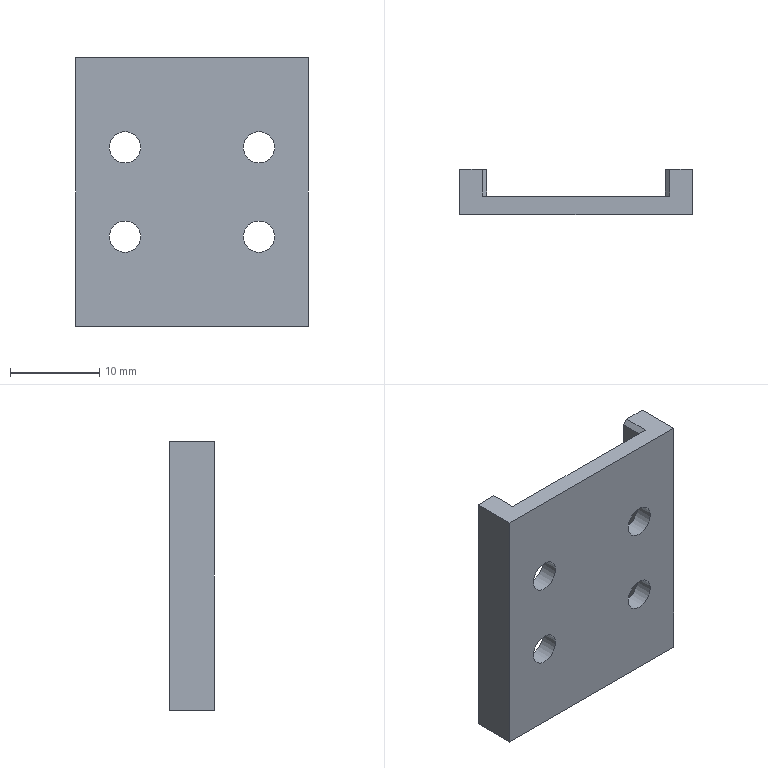NC program | NX | posted with a generic post | part box 26 x 5 x 30 mm
Whole program:
N10 G17 G21 G94 G90
(FLOOR_WALL , TOOL : D50)
N12 T01 M6
N14 G54
N16 G17 G0 G90 X-43. Y0. B0. C0. S2000 M3
N18 G43 Z30. H1
N20 Z3.
N22 G94 G1 Z0. F800.
N24 X-40.
N26 X40.
N28 X43.
N30 Z3.
N32 G0 Z30.
N34 M5
(DRILLING , TOOL : ZXZ)
N36 T02 M6
N38 G54
N40 G17 G0 G90 X-5. Y7.5 B0. C0. S3500 M3
N42 G43 Z30. H2
N44 G94 G81 G98 Z-1. F250. R3.
N46 X5.
N48 Y-7.5
N50 X-5.
N52 G80
N54 G0 X-5. Y-7.5 Z30.
N56 M5
(DRILLING_COPY , TOOL : 3.5ZT)
N58 T13 M6
N60 G54
N62 G17 G0 G90 X-5. Y7.5 B0. C0. S2000 M3
N64 G43 Z30. H13
N66 G94 G83 G98 Z-7.552 F150. Q2. R3.
N68 X5.
N70 Y-7.5
N72 X-5.
N74 G80
N76 G0 X-5. Y-7.5 Z30.
N78 M5
(FLOOR_WALL_1 , TOOL : D10)
N80 T10 M6
N82 G54
N84 G17 G0 G90 X-21.5 Y-1.443 B0. C0. S3000 M3
N86 G43 Z30. H10
N88 Z0.924
N90 G94 G1 Z-0.076 F1000.
N92 X-20.5 Y-0.866
N94 G3 X-20. Y0. R1.
N96 G1 Y8.358 F2000.
N98 X-16.592 Y4.95
N100 X16.592
N102 X20. Y8.358
N104 Y-8.358
N106 X16.592 Y-4.95
N108 X-16.592
N110 X-20. Y-8.358
N112 Y0.
N114 X-15.5
N116 Y0.45
N118 X15.5
N120 Y-0.45
N122 X-15.5
N124 Y0.
N126 G3 X-16. Y0.866 R1.
N128 G1 Z0.924
N130 G0 X-21.5 Y-1.443 Z0.734
N132 G1 Z-0.266 F1000.
N134 X-20.5 Y-0.866
N136 G3 X-20. Y0. R1.
N138 G1 Y8.358 F2000.
N140 X-16.592 Y4.95
N142 X16.592
N144 X20. Y8.358
N146 Y-8.358
N148 X16.592 Y-4.95
N150 X-16.592
N152 X-20. Y-8.358
N154 Y0.
N156 X-15.5
N158 Y0.45
N160 X15.5
N162 Y-0.45
N164 X-15.5
N166 Y0.
N168 G3 X-16. Y0.866 R1.
N170 G1 Z0.734
N172 G0 X-21.5 Y-1.443 Z0.543
N174 G1 Z-0.457 F1000.
N176 X-20.5 Y-0.866
N178 G3 X-20. Y0. R1.
N180 G1 Y8.358 F2000.
N182 X-16.592 Y4.95
N184 X16.592
N186 X20. Y8.358
N188 Y-8.358
N190 X16.592 Y-4.95
N192 X-16.592
N194 X-20. Y-8.358
N196 Y0.
N198 X-15.5
N200 Y0.45
N202 X15.5
N204 Y-0.45
N206 X-15.5
N208 Y0.
N210 G3 X-16. Y0.866 R1.
N212 G1 Z0.543
N214 G0 X-21.5 Y-1.443 Z0.353
N216 G1 Z-0.648 F1000.
N218 X-20.5 Y-0.866
N220 G3 X-20. Y0. R1.
N222 G1 Y8.358 F2000.
N224 X-16.592 Y4.95
N226 X16.592
N228 X20. Y8.358
N230 Y-8.358
N232 X16.592 Y-4.95
N234 X-16.592
N236 X-20. Y-8.358
N238 Y0.
N240 X-15.5
N242 Y0.45
N244 X15.5
N246 Y-0.45
N248 X-15.5
N250 Y0.
N252 G3 X-16. Y0.866 R1.
N254 G1 Z0.353
N256 G0 X-21.5 Y-1.443 Z0.162
N258 G1 Z-0.838 F1000.
N260 X-20.5 Y-0.866
N262 G3 X-20. Y0. R1.
N264 G1 Y8.358 F2000.
N266 X-16.592 Y4.95
N268 X16.592
N270 X20. Y8.358
N272 Y-8.358
N274 X16.592 Y-4.95
N276 X-16.592
N278 X-20. Y-8.358
N280 Y0.
N282 X-15.5
N284 Y0.45
N286 X15.5
N288 Y-0.45
N290 X-15.5
N292 Y0.
N294 G3 X-16. Y0.866 R1.
N296 G1 Z0.162
N298 G0 X-21.5 Y-1.443 Z-0.029
N300 G1 Z-1.029 F1000.
N302 X-20.5 Y-0.866
N304 G3 X-20. Y0. R1.
N306 G1 Y8.358 F2000.
N308 X-16.592 Y4.95
N310 X16.592
N312 X20. Y8.358
N314 Y-8.358
N316 X16.592 Y-4.95
N318 X-16.592
N320 X-20. Y-8.358
N322 Y0.
N324 X-15.5
N326 Y0.45
N328 X15.5
N330 Y-0.45
N332 X-15.5
N334 Y0.
N336 G3 X-16. Y0.866 R1.
N338 G1 Z-0.029
N340 G0 X-21.5 Y-1.443 Z-0.219
N342 G1 Z-1.219 F1000.
N344 X-20.5 Y-0.866
N346 G3 X-20. Y0. R1.
N348 G1 Y8.358 F2000.
N350 X-16.592 Y4.95
N352 X16.592
N354 X20. Y8.358
N356 Y-8.358
N358 X16.592 Y-4.95
N360 X-16.592
N362 X-20. Y-8.358
N364 Y0.
N366 X-15.5
N368 Y0.45
N370 X15.5
N372 Y-0.45
N374 X-15.5
N376 Y0.
N378 G3 X-16. Y0.866 R1.
N380 G1 Z-0.219
N382 G0 X-21.5 Y-1.443 Z-0.41
N384 G1 Z-1.41 F1000.
N386 X-20.5 Y-0.866
N388 G3 X-20. Y0. R1.
N390 G1 Y8.358 F2000.
N392 X-16.592 Y4.95
N394 X16.592
N396 X20. Y8.358
N398 Y-8.358
N400 X16.592 Y-4.95
N402 X-16.592
N404 X-20. Y-8.358
N406 Y0.
N408 X-15.5
N410 Y0.45
N412 X15.5
N414 Y-0.45
N416 X-15.5
N418 Y0.
N420 G3 X-16. Y0.866 R1.
N422 G1 Z-0.41
N424 G0 X-21.5 Y-1.443 Z-0.601
N426 G1 Z-1.601 F1000.
N428 X-20.5 Y-0.866
N430 G3 X-20. Y0. R1.
N432 G1 Y8.358 F2000.
N434 X-16.592 Y4.95
N436 X16.592
N438 X20. Y8.358
N440 Y-8.358
N442 X16.592 Y-4.95
N444 X-16.592
N446 X-20. Y-8.358
N448 Y0.
N450 X-15.5
N452 Y0.45
N454 X15.5
N456 Y-0.45
N458 X-15.5
N460 Y0.
N462 G3 X-16. Y0.866 R1.
N464 G1 Z-0.601
N466 G0 X-21.5 Y-1.443 Z-0.791
N468 G1 Z-1.791 F1000.
N470 X-20.5 Y-0.866
N472 G3 X-20. Y0. R1.
N474 G1 Y8.358 F2000.
N476 X-16.592 Y4.95
N478 X16.592
N480 X20. Y8.358
N482 Y-8.358
N484 X16.592 Y-4.95
N486 X-16.592
N488 X-20. Y-8.358
N490 Y0.
N492 X-15.5
N494 Y0.45
N496 X15.5
N498 Y-0.45
N500 X-15.5
N502 Y0.
N504 G3 X-16. Y0.866 R1.
N506 G1 Z-0.791
N508 G0 X-21.5 Y-1.443 Z-0.982
N510 G1 Z-1.982 F1000.
N512 X-20.5 Y-0.866
N514 G3 X-20. Y0. R1.
N516 G1 Y8.358 F2000.
N518 X-16.592 Y4.95
N520 X16.592
N522 X20. Y8.358
N524 Y-8.358
N526 X16.592 Y-4.95
N528 X-16.592
N530 X-20. Y-8.358
N532 Y0.
N534 X-15.5
N536 Y0.45
N538 X15.5
N540 Y-0.45
N542 X-15.5
N544 Y0.
N546 G3 X-16. Y0.866 R1.
N548 G1 Z-0.982
N550 G0 X-21.5 Y-1.443 Z-1.173
N552 G1 Z-2.173 F1000.
N554 X-20.5 Y-0.866
N556 G3 X-20. Y0. R1.
N558 G1 Y8.358 F2000.
N560 X-16.592 Y4.95
N562 X16.592
N564 X20. Y8.358
N566 Y-8.358
N568 X16.592 Y-4.95
N570 X-16.592
N572 X-20. Y-8.358
N574 Y0.
N576 X-15.5
N578 Y0.45
N580 X15.5
N582 Y-0.45
N584 X-15.5
N586 Y0.
N588 G3 X-16. Y0.866 R1.
N590 G1 Z-1.173
N592 G0 X-21.5 Y-1.443 Z-1.363
N594 G1 Z-2.363 F1000.
N596 X-20.5 Y-0.866
N598 G3 X-20. Y0. R1.
N600 G1 Y8.358 F2000.
N602 X-16.592 Y4.95
N604 X16.592
N606 X20. Y8.358
N608 Y-8.358
N610 X16.592 Y-4.95
N612 X-16.592
N614 X-20. Y-8.358
N616 Y0.
N618 X-15.5
N620 Y0.45
N622 X15.5
N624 Y-0.45
N626 X-15.5
N628 Y0.
N630 G3 X-16. Y0.866 R1.
N632 G1 Z-1.363
N634 G0 X-21.5 Y-1.443 Z-1.554
N636 G1 Z-2.554 F1000.
N638 X-20.5 Y-0.866
N640 G3 X-20. Y0. R1.
N642 G1 Y8.358 F2000.
N644 X-16.592 Y4.95
N646 X16.592
N648 X20. Y8.358
N650 Y-8.358
N652 X16.592 Y-4.95
N654 X-16.592
N656 X-20. Y-8.358
N658 Y0.
N660 X-15.5
N662 Y0.45
N664 X15.5
N666 Y-0.45
N668 X-15.5
N670 Y0.
N672 G3 X-16. Y0.866 R1.
N674 G1 Z-1.554
N676 G0 X-21.5 Y-1.443 Z-1.744
N678 G1 Z-2.744 F1000.
N680 X-20.5 Y-0.866
N682 G3 X-20. Y0. R1.
N684 G1 Y8.358 F2000.
N686 X-16.592 Y4.95
N688 X16.592
N690 X20. Y8.358
N692 Y-8.358
N694 X16.592 Y-4.95
N696 X-16.592
N698 X-20. Y-8.358
N700 Y0.
N702 X-15.5
N704 Y0.45
N706 X15.5
N708 Y-0.45
N710 X-15.5
N712 Y0.
N714 G3 X-16. Y0.866 R1.
N716 G1 Z-1.744
N718 G0 X-21.5 Y-1.443 Z-1.935
N720 G1 Z-2.935 F1000.
N722 X-20.5 Y-0.866
N724 G3 X-20. Y0. R1.
N726 G1 Y8.358 F2000.
N728 X-16.592 Y4.95
N730 X16.592
N732 X20. Y8.358
N734 Y-8.358
N736 X16.592 Y-4.95
N738 X-16.592
N740 X-20. Y-8.358
N742 Y0.
N744 X-15.5
N746 Y0.45
N748 X15.5
N750 Y-0.45
N752 X-15.5
N754 Y0.
N756 G3 X-16. Y0.866 R1.
N758 G1 Z-1.935
N760 G0 Z30.
N762 M5
(FLOOR_WALL_1_COPY , TOOL : D6JING)
N764 T06 M6
N766 G54
N768 G17 G0 G90 X-19.5 Y8.697 B0. C0. S6000 M3
N770 G43 Z30. H6
N772 Z-1.985
N774 G94 G1 Z-2.985 F1000.
N776 X-18.52 Y6.999
N778 G3 X-18. Y6.699 R0.6
N780 G1 X18.
N782 Y4.019
N784 X-18.
N786 Y1.339
N788 X18.
N790 Y-1.34
N792 X-18.
N794 Y-4.02
N796 X18.
N798 Y-6.7
N800 X-18.
N802 G2 X-18.52 Y-6.4 R0.6
N804 G1 X-19.5 Y-4.702
N806 Z-1.985
N808 Y-9.166 F8000.
N810 Z-2.985 F1000.
N812 X-18.58 Y-9.413
N814 G3 X-18. Y-9.257 R0.6
N816 G1 X-15.743 Y-7.
N818 X15.743
N820 X18. Y-9.257
N822 G3 X18.58 Y-9.413 R0.6
N824 G1 X19.5 Y-9.166
N826 Z-1.985
N828 Y9.166 F8000.
N830 Z-2.985 F1000.
N832 X18.58 Y9.413
N834 G3 X18. Y9.257 R0.6
N836 G1 X15.743 Y7.
N838 X-15.743
N840 X-18. Y9.257
N842 G3 X-18.58 Y9.413 R0.6
N844 G1 X-19.5 Y9.166
N846 Z-1.985
N848 G0 Z30.
N850 M5
(PLANAR_MILL , TOOL : D4A45)
N852 T07 M6
N854 G54
N856 G17 G0 G90 X1.039 Y-14.5 B0. C0. S7500 M3
N858 G43 Z30. H7
N860 Z0.5
N862 G94 G1 Z-1. F1250.
N864 X0.866 Y-14.2
N866 G3 X0. Y-13.7 R1.
N868 G1 X-14.7
N870 G2 X-15.7 Y-12.7 R1.
N872 G1 Y-10.624
N874 G2 X-15.407 Y-9.917 R1.
N876 G1 X-15.083 Y-9.593
N878 G2 X-14.376 Y-9.3 R1.
N880 G1 X14.376
N882 G2 X15.083 Y-9.593 R1.
N884 G1 X15.407 Y-9.917
N886 G2 X15.7 Y-10.624 R1.
N888 G1 Y-12.7
N890 G2 X14.7 Y-13.7 R1.
N892 G1 X0.
N894 G3 X-0.866 Y-14.2 R1.
N896 G1 X-1.039 Y-14.5
N898 Z0.5
N900 G0 Z30.
N902 Y14.5
N904 Z0.5
N906 G1 Z-1.
N908 X-0.866 Y14.2
N910 G3 X0. Y13.7 R1.
N912 G1 X14.7
N914 G2 X15.7 Y12.7 R1.
N916 G1 Y10.624
N918 G2 X15.407 Y9.917 R1.
N920 G1 X15.083 Y9.593
N922 G2 X14.376 Y9.3 R1.
N924 G1 X-14.376
N926 G2 X-15.083 Y9.593 R1.
N928 G1 X-15.407 Y9.917
N930 G2 X-15.7 Y10.624 R1.
N932 G1 Y12.7
N934 G2 X-14.7 Y13.7 R1.
N936 G1 X0.
N938 G3 X0.866 Y14.2 R1.
N940 G1 X1.039 Y14.5
N942 Z0.5
N944 G0 Z30.
(PLANAR_MILL_COPY , TOOL : D4A45)
N946 X-16.856 Y-7.689
N948 Z-2.485
N950 G1 Z-3.985
N952 X-16.7 Y-7.784
N954 G3 X-15.7 Y-7.807 R1.
N956 G1 Y7.807
N958 G3 X-16.7 Y7.784 R1.
N960 G1 X-16.856 Y7.689
N962 Z-2.485
N964 G0 Z30.
N966 X16.856
N968 Z-2.485
N970 G1 Z-3.985
N972 X16.7 Y7.784
N974 G3 X15.7 Y7.807 R1.
N976 G1 Y-7.807
N978 G3 X16.7 Y-7.784 R1.
N980 G1 X16.856 Y-7.689
N982 Z-2.485
N984 G0 Z30.
(DRILLING_COPY_1 , TOOL : D4A45)
N986 X-5. Y7.5 S3500
N988 G81 G98 Z-4.885 F250. R0.015
N990 X5.
N992 Y-7.5
N994 X-5.
N996 G80
N998 G0 X-5. Y-7.5 Z30.
N1000 M5
(刀补 , TOOL : D6JING)
N1002 T06 M6
N1004 G54
N1006 G17 G0 G90 X-19.591 Y-9.124 B0. C0. S6000 M3
N1008 G43 Z30. H6
N1010 Z-1.985
N1012 G94 G1 Z-2.985 F1000.
N1014 G41 X-19.5 Y-9.166 D6
N1016 X-18.58 Y-9.413
N1018 G3 X-18. Y-9.257 R0.6
N1020 G1 X-15.743 Y-7.
N1022 X15.743
N1024 X18. Y-9.257
N1026 G3 X18.58 Y-9.413 R0.6
N1028 G1 X19.5 Y-9.166
N1030 G40
N1032 X19.591 Y-9.124
N1034 Z-1.985
N1036 Y9.124 F8000.
N1038 Z-2.985 F1000.
N1040 G41 X19.5 Y9.166
N1042 X18.58 Y9.413
N1044 G3 X18. Y9.257 R0.6
N1046 G1 X15.743 Y7.
N1048 X-15.743
N1050 X-18. Y9.257
N1052 G3 X-18.58 Y9.413 R0.6
N1054 G1 X-19.5 Y9.166
N1056 G40
N1058 X-19.591 Y9.124
N1060 Z-1.985
N1062 G0 Z30.
N1064 M5
N1066 M2